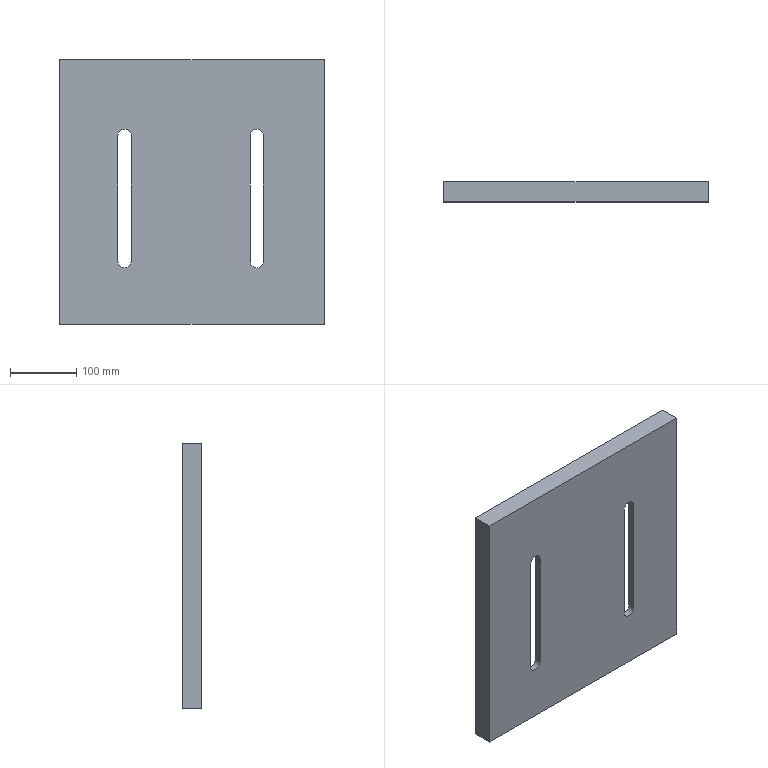Part | STEP file | leg control03_5 | 1 solid | 21 faces | box 400 x 30 x 400 mm | volume 2067797 mm3 | plane 15 | cylinder 6 | commonest cylinder face diameters 20 x6